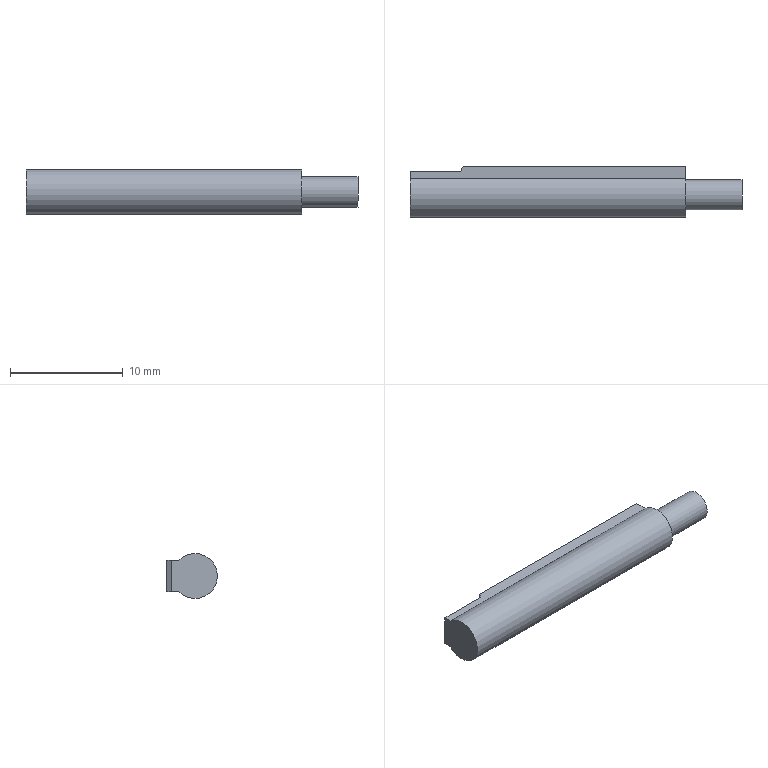Part | NX | 1 solid | 23 faces | box 29.5 x 4.5 x 4 mm | volume 373.823 mm3 | plane 19 | cylinder 4 | commonest cylinder face diameters 2 x1 2.5 x1 2.7 x1 4 x1
STEP:
#1=CARTESIAN_POINT('',(2.462,2.1,-0.8867));
#2=VERTEX_POINT('',#1);
#3=CARTESIAN_POINT('',(1.113,2.1,0.4624));
#4=VERTEX_POINT('',#3);
#5=CARTESIAN_POINT('',(2.,2.1,0.));
#6=DIRECTION('',(0.,1.,0.));
#7=DIRECTION('',(0.,0.,1.));
#8=AXIS2_PLACEMENT_3D('',#5,#6,#7);
#9=CIRCLE('',#8,1.);
#10=EDGE_CURVE('',#2,#4,#9,.T.);
#11=ORIENTED_EDGE('',*,*,#10,.T.);
#12=CARTESIAN_POINT('',(13.738,2.1,-12.162));
#13=DIRECTION('',(0.7071,0.,-0.7071));
#14=VECTOR('',#13,1000.);
#15=LINE('',#12,#14);
#16=EDGE_CURVE('',#4,#2,#15,.T.);
#17=ORIENTED_EDGE('',*,*,#16,.T.);
#18=EDGE_LOOP('',(#11,#17));
#19=FACE_BOUND('',#18,.T.);
#20=CARTESIAN_POINT('',(24.5,2.1,-1.4));
#21=DIRECTION('',(0.,-1.,0.));
#22=DIRECTION('',(0.,0.,-1.));
#23=AXIS2_PLACEMENT_3D('',#20,#21,#22);
#24=PLANE('',#23);
#25=ADVANCED_FACE('',(#19),#24,.F.);
#26=CARTESIAN_POINT('',(24.5,1.428,1.4));
#27=VERTEX_POINT('',#26);
#28=CARTESIAN_POINT('',(24.5,1.428,-1.4));
#29=VERTEX_POINT('',#28);
#30=CARTESIAN_POINT('',(24.5,0.,0.));
#31=DIRECTION('',(1.,0.,0.));
#32=DIRECTION('',(0.,0.,-1.));
#33=AXIS2_PLACEMENT_3D('',#30,#31,#32);
#34=CIRCLE('',#33,2.);
#35=EDGE_CURVE('',#27,#29,#34,.T.);
#36=ORIENTED_EDGE('',*,*,#35,.T.);
#37=CARTESIAN_POINT('',(24.5,2.5,-1.4));
#38=VERTEX_POINT('',#37);
#39=CARTESIAN_POINT('',(24.5,1.428,-1.4));
#40=DIRECTION('',(0.,1.,0.));
#41=VECTOR('',#40,1000.);
#42=LINE('',#39,#41);
#43=EDGE_CURVE('',#29,#38,#42,.T.);
#44=ORIENTED_EDGE('',*,*,#43,.T.);
#45=CARTESIAN_POINT('',(24.5,2.5,1.4));
#46=VERTEX_POINT('',#45);
#47=CARTESIAN_POINT('',(24.5,2.5,1.4));
#48=DIRECTION('',(0.,0.,-1.));
#49=VECTOR('',#48,1000.);
#50=LINE('',#47,#49);
#51=EDGE_CURVE('',#46,#38,#50,.T.);
#52=ORIENTED_EDGE('',*,*,#51,.F.);
#53=CARTESIAN_POINT('',(24.5,2.1,1.4));
#54=DIRECTION('',(0.,-1.,0.));
#55=VECTOR('',#54,1000.);
#56=LINE('',#53,#55);
#57=EDGE_CURVE('',#46,#27,#56,.T.);
#58=ORIENTED_EDGE('',*,*,#57,.T.);
#59=EDGE_LOOP('',(#36,#44,#52,#58));
#60=FACE_BOUND('',#59,.T.);
#61=CARTESIAN_POINT('',(24.5,0.,-1.35));
#62=VERTEX_POINT('',#61);
#63=CARTESIAN_POINT('',(24.5,0.,0.));
#64=DIRECTION('',(1.,0.,0.));
#65=DIRECTION('',(0.,0.,-1.));
#66=AXIS2_PLACEMENT_3D('',#63,#64,#65);
#67=CIRCLE('',#66,1.35);
#68=EDGE_CURVE('',#62,#62,#67,.F.);
#69=ORIENTED_EDGE('',*,*,#68,.T.);
#70=EDGE_LOOP('',(#69));
#71=FACE_BOUND('',#70,.T.);
#72=CARTESIAN_POINT('',(24.5,0.,0.));
#73=DIRECTION('',(1.,0.,0.));
#74=DIRECTION('',(0.,0.,-1.));
#75=AXIS2_PLACEMENT_3D('',#72,#73,#74);
#76=PLANE('',#75);
#77=ADVANCED_FACE('',(#60,#71),#76,.T.);
#78=CARTESIAN_POINT('',(0.,1.428,1.4));
#79=VERTEX_POINT('',#78);
#80=CARTESIAN_POINT('',(0.,1.428,-1.4));
#81=VERTEX_POINT('',#80);
#82=CARTESIAN_POINT('',(0.,0.,0.));
#83=DIRECTION('',(1.,0.,0.));
#84=DIRECTION('',(0.,0.,-1.));
#85=AXIS2_PLACEMENT_3D('',#82,#83,#84);
#86=CIRCLE('',#85,2.);
#87=EDGE_CURVE('',#79,#81,#86,.T.);
#88=ORIENTED_EDGE('',*,*,#87,.T.);
#89=CARTESIAN_POINT('',(24.5,1.428,-1.4));
#90=DIRECTION('',(-1.,0.,0.));
#91=VECTOR('',#90,1000.);
#92=LINE('',#89,#91);
#93=EDGE_CURVE('',#29,#81,#92,.T.);
#94=ORIENTED_EDGE('',*,*,#93,.F.);
#95=ORIENTED_EDGE('',*,*,#35,.F.);
#96=CARTESIAN_POINT('',(24.5,1.428,1.4));
#97=DIRECTION('',(-1.,0.,0.));
#98=VECTOR('',#97,1000.);
#99=LINE('',#96,#98);
#100=EDGE_CURVE('',#27,#79,#99,.T.);
#101=ORIENTED_EDGE('',*,*,#100,.T.);
#102=EDGE_LOOP('',(#88,#94,#95,#101));
#103=FACE_BOUND('',#102,.T.);
#104=CARTESIAN_POINT('',(24.5,0.,0.));
#105=DIRECTION('',(-1.,0.,0.));
#106=DIRECTION('',(0.,0.,1.));
#107=AXIS2_PLACEMENT_3D('',#104,#105,#106);
#108=CYLINDRICAL_SURFACE('',#107,2.);
#109=ADVANCED_FACE('',(#103),#108,.T.);
#110=CARTESIAN_POINT('',(0.,2.1,-1.4));
#111=VERTEX_POINT('',#110);
#112=CARTESIAN_POINT('',(0.,1.428,-1.4));
#113=DIRECTION('',(0.,1.,0.));
#114=VECTOR('',#113,1000.);
#115=LINE('',#112,#114);
#116=EDGE_CURVE('',#81,#111,#115,.T.);
#117=ORIENTED_EDGE('',*,*,#116,.T.);
#118=CARTESIAN_POINT('',(4.5,2.1,-1.4));
#119=VERTEX_POINT('',#118);
#120=CARTESIAN_POINT('',(24.5,2.1,-1.4));
#121=DIRECTION('',(-1.,0.,0.));
#122=VECTOR('',#121,1000.);
#123=LINE('',#120,#122);
#124=EDGE_CURVE('',#119,#111,#123,.T.);
#125=ORIENTED_EDGE('',*,*,#124,.F.);
#126=CARTESIAN_POINT('',(4.731,2.5,-1.4));
#127=VERTEX_POINT('',#126);
#128=CARTESIAN_POINT('',(4.731,2.5,-1.4));
#129=DIRECTION('',(-0.5,-0.866,0.));
#130=VECTOR('',#129,1000.);
#131=LINE('',#128,#130);
#132=EDGE_CURVE('',#127,#119,#131,.T.);
#133=ORIENTED_EDGE('',*,*,#132,.F.);
#134=CARTESIAN_POINT('',(24.5,2.5,-1.4));
#135=DIRECTION('',(-1.,0.,0.));
#136=VECTOR('',#135,1000.);
#137=LINE('',#134,#136);
#138=EDGE_CURVE('',#38,#127,#137,.T.);
#139=ORIENTED_EDGE('',*,*,#138,.F.);
#140=ORIENTED_EDGE('',*,*,#43,.F.);
#141=ORIENTED_EDGE('',*,*,#93,.T.);
#142=EDGE_LOOP('',(#117,#125,#133,#139,#140,#141));
#143=FACE_BOUND('',#142,.T.);
#144=CARTESIAN_POINT('',(24.5,1.428,-1.4));
#145=DIRECTION('',(0.,0.,1.));
#146=DIRECTION('',(1.,0.,0.));
#147=AXIS2_PLACEMENT_3D('',#144,#145,#146);
#148=PLANE('',#147);
#149=ADVANCED_FACE('',(#143),#148,.F.);
#150=CARTESIAN_POINT('',(2.,2.1,1.25));
#151=VERTEX_POINT('',#150);
#152=CARTESIAN_POINT('',(2.,2.1,0.));
#153=DIRECTION('',(0.,1.,0.));
#154=DIRECTION('',(0.,0.,1.));
#155=AXIS2_PLACEMENT_3D('',#152,#153,#154);
#156=CIRCLE('',#155,1.25);
#157=EDGE_CURVE('',#151,#151,#156,.T.);
#158=ORIENTED_EDGE('',*,*,#157,.F.);
#159=EDGE_LOOP('',(#158));
#160=FACE_BOUND('',#159,.T.);
#161=CARTESIAN_POINT('',(4.5,2.1,1.4));
#162=VERTEX_POINT('',#161);
#163=CARTESIAN_POINT('',(0.,2.1,1.4));
#164=VERTEX_POINT('',#163);
#165=CARTESIAN_POINT('',(24.5,2.1,1.4));
#166=DIRECTION('',(-1.,0.,0.));
#167=VECTOR('',#166,1000.);
#168=LINE('',#165,#167);
#169=EDGE_CURVE('',#162,#164,#168,.T.);
#170=ORIENTED_EDGE('',*,*,#169,.F.);
#171=CARTESIAN_POINT('',(4.5,2.1,1.4));
#172=DIRECTION('',(0.,0.,-1.));
#173=VECTOR('',#172,1000.);
#174=LINE('',#171,#173);
#175=EDGE_CURVE('',#162,#119,#174,.T.);
#176=ORIENTED_EDGE('',*,*,#175,.T.);
#177=ORIENTED_EDGE('',*,*,#124,.T.);
#178=CARTESIAN_POINT('',(0.,2.1,-1.4));
#179=DIRECTION('',(0.,0.,1.));
#180=VECTOR('',#179,1000.);
#181=LINE('',#178,#180);
#182=EDGE_CURVE('',#111,#164,#181,.T.);
#183=ORIENTED_EDGE('',*,*,#182,.T.);
#184=EDGE_LOOP('',(#170,#176,#177,#183));
#185=FACE_BOUND('',#184,.T.);
#186=CARTESIAN_POINT('',(24.5,2.1,-1.4));
#187=DIRECTION('',(0.,-1.,0.));
#188=DIRECTION('',(0.,0.,-1.));
#189=AXIS2_PLACEMENT_3D('',#186,#187,#188);
#190=PLANE('',#189);
#191=ADVANCED_FACE('',(#160,#185),#190,.F.);
#192=CARTESIAN_POINT('',(0.,2.1,1.4));
#193=DIRECTION('',(0.,-1.,0.));
#194=VECTOR('',#193,1000.);
#195=LINE('',#192,#194);
#196=EDGE_CURVE('',#164,#79,#195,.T.);
#197=ORIENTED_EDGE('',*,*,#196,.T.);
#198=ORIENTED_EDGE('',*,*,#100,.F.);
#199=ORIENTED_EDGE('',*,*,#57,.F.);
#200=CARTESIAN_POINT('',(4.731,2.5,1.4));
#201=VERTEX_POINT('',#200);
#202=CARTESIAN_POINT('',(24.5,2.5,1.4));
#203=DIRECTION('',(-1.,0.,0.));
#204=VECTOR('',#203,1000.);
#205=LINE('',#202,#204);
#206=EDGE_CURVE('',#46,#201,#205,.T.);
#207=ORIENTED_EDGE('',*,*,#206,.T.);
#208=CARTESIAN_POINT('',(4.731,2.5,1.4));
#209=DIRECTION('',(-0.5,-0.866,0.));
#210=VECTOR('',#209,1000.);
#211=LINE('',#208,#210);
#212=EDGE_CURVE('',#201,#162,#211,.T.);
#213=ORIENTED_EDGE('',*,*,#212,.T.);
#214=ORIENTED_EDGE('',*,*,#169,.T.);
#215=EDGE_LOOP('',(#197,#198,#199,#207,#213,#214));
#216=FACE_BOUND('',#215,.T.);
#217=CARTESIAN_POINT('',(24.5,2.1,1.4));
#218=DIRECTION('',(0.,0.,-1.));
#219=DIRECTION('',(-1.,0.,0.));
#220=AXIS2_PLACEMENT_3D('',#217,#218,#219);
#221=PLANE('',#220);
#222=ADVANCED_FACE('',(#216),#221,.F.);
#223=ORIENTED_EDGE('',*,*,#87,.F.);
#224=ORIENTED_EDGE('',*,*,#196,.F.);
#225=ORIENTED_EDGE('',*,*,#182,.F.);
#226=ORIENTED_EDGE('',*,*,#116,.F.);
#227=EDGE_LOOP('',(#223,#224,#225,#226));
#228=FACE_BOUND('',#227,.T.);
#229=CARTESIAN_POINT('',(0.,0.,0.));
#230=DIRECTION('',(1.,0.,0.));
#231=DIRECTION('',(0.,0.,-1.));
#232=AXIS2_PLACEMENT_3D('',#229,#230,#231);
#233=PLANE('',#232);
#234=ADVANCED_FACE('',(#228),#233,.F.);
#235=ORIENTED_EDGE('',*,*,#68,.F.);
#236=EDGE_LOOP('',(#235));
#237=FACE_BOUND('',#236,.T.);
#238=CARTESIAN_POINT('',(29.5,0.,-1.35));
#239=VERTEX_POINT('',#238);
#240=CARTESIAN_POINT('',(29.5,0.,0.));
#241=DIRECTION('',(1.,0.,0.));
#242=DIRECTION('',(0.,0.,-1.));
#243=AXIS2_PLACEMENT_3D('',#240,#241,#242);
#244=CIRCLE('',#243,1.35);
#245=EDGE_CURVE('',#239,#239,#244,.T.);
#246=ORIENTED_EDGE('',*,*,#245,.F.);
#247=EDGE_LOOP('',(#246));
#248=FACE_BOUND('',#247,.T.);
#249=CARTESIAN_POINT('',(29.5,0.,0.));
#250=DIRECTION('',(-1.,0.,0.));
#251=DIRECTION('',(0.,0.,1.));
#252=AXIS2_PLACEMENT_3D('',#249,#250,#251);
#253=CYLINDRICAL_SURFACE('',#252,1.35);
#254=ADVANCED_FACE('',(#237,#248),#253,.T.);
#255=ORIENTED_EDGE('',*,*,#245,.T.);
#256=EDGE_LOOP('',(#255));
#257=FACE_BOUND('',#256,.T.);
#258=CARTESIAN_POINT('',(29.5,0.,0.));
#259=DIRECTION('',(1.,0.,0.));
#260=DIRECTION('',(0.,0.,-1.));
#261=AXIS2_PLACEMENT_3D('',#258,#259,#260);
#262=PLANE('',#261);
#263=ADVANCED_FACE('',(#257),#262,.T.);
#264=CARTESIAN_POINT('',(2.,0.6,1.25));
#265=VERTEX_POINT('',#264);
#266=CARTESIAN_POINT('',(2.,0.6,0.));
#267=DIRECTION('',(0.,1.,0.));
#268=DIRECTION('',(0.,0.,1.));
#269=AXIS2_PLACEMENT_3D('',#266,#267,#268);
#270=CIRCLE('',#269,1.25);
#271=EDGE_CURVE('',#265,#265,#270,.T.);
#272=ORIENTED_EDGE('',*,*,#271,.F.);
#273=EDGE_LOOP('',(#272));
#274=FACE_BOUND('',#273,.T.);
#275=ORIENTED_EDGE('',*,*,#157,.T.);
#276=EDGE_LOOP('',(#275));
#277=FACE_BOUND('',#276,.T.);
#278=CARTESIAN_POINT('',(2.,0.6,0.));
#279=DIRECTION('',(0.,1.,0.));
#280=DIRECTION('',(0.,0.,1.));
#281=AXIS2_PLACEMENT_3D('',#278,#279,#280);
#282=CYLINDRICAL_SURFACE('',#281,1.25);
#283=ADVANCED_FACE('',(#274,#277),#282,.F.);
#284=CARTESIAN_POINT('',(2.,0.6,1.));
#285=VERTEX_POINT('',#284);
#286=CARTESIAN_POINT('',(2.,0.6,0.));
#287=DIRECTION('',(0.,1.,0.));
#288=DIRECTION('',(0.,0.,1.));
#289=AXIS2_PLACEMENT_3D('',#286,#287,#288);
#290=CIRCLE('',#289,1.);
#291=EDGE_CURVE('',#285,#285,#290,.T.);
#292=ORIENTED_EDGE('',*,*,#291,.F.);
#293=EDGE_LOOP('',(#292));
#294=FACE_BOUND('',#293,.T.);
#295=ORIENTED_EDGE('',*,*,#271,.T.);
#296=EDGE_LOOP('',(#295));
#297=FACE_BOUND('',#296,.T.);
#298=CARTESIAN_POINT('',(2.,0.6,0.));
#299=DIRECTION('',(0.,1.,0.));
#300=DIRECTION('',(0.,0.,1.));
#301=AXIS2_PLACEMENT_3D('',#298,#299,#300);
#302=PLANE('',#301);
#303=ADVANCED_FACE('',(#294,#297),#302,.T.);
#304=CARTESIAN_POINT('',(1.113,1.1,0.4624));
#305=VERTEX_POINT('',#304);
#306=CARTESIAN_POINT('',(1.113,0.6,0.4624));
#307=DIRECTION('',(0.,1.,0.));
#308=VECTOR('',#307,1000.);
#309=LINE('',#306,#308);
#310=EDGE_CURVE('',#4,#305,#309,.F.);
#311=ORIENTED_EDGE('',*,*,#310,.F.);
#312=ORIENTED_EDGE('',*,*,#10,.F.);
#313=CARTESIAN_POINT('',(2.462,1.1,-0.8867));
#314=VERTEX_POINT('',#313);
#315=CARTESIAN_POINT('',(2.462,0.6,-0.8867));
#316=DIRECTION('',(0.,1.,0.));
#317=VECTOR('',#316,1000.);
#318=LINE('',#315,#317);
#319=EDGE_CURVE('',#314,#2,#318,.T.);
#320=ORIENTED_EDGE('',*,*,#319,.F.);
#321=CARTESIAN_POINT('',(2.887,1.1,-0.4624));
#322=VERTEX_POINT('',#321);
#323=CARTESIAN_POINT('',(2.,1.1,0.));
#324=DIRECTION('',(0.,1.,0.));
#325=DIRECTION('',(0.,0.,1.));
#326=AXIS2_PLACEMENT_3D('',#323,#324,#325);
#327=CIRCLE('',#326,1.);
#328=EDGE_CURVE('',#314,#322,#327,.F.);
#329=ORIENTED_EDGE('',*,*,#328,.T.);
#330=CARTESIAN_POINT('',(2.887,2.1,-0.4624));
#331=VERTEX_POINT('',#330);
#332=CARTESIAN_POINT('',(2.887,0.6,-0.4624));
#333=DIRECTION('',(0.,1.,0.));
#334=VECTOR('',#333,1000.);
#335=LINE('',#332,#334);
#336=EDGE_CURVE('',#331,#322,#335,.F.);
#337=ORIENTED_EDGE('',*,*,#336,.F.);
#338=CARTESIAN_POINT('',(1.538,2.1,0.8867));
#339=VERTEX_POINT('',#338);
#340=CARTESIAN_POINT('',(2.,2.1,0.));
#341=DIRECTION('',(0.,1.,0.));
#342=DIRECTION('',(0.,0.,1.));
#343=AXIS2_PLACEMENT_3D('',#340,#341,#342);
#344=CIRCLE('',#343,1.);
#345=EDGE_CURVE('',#339,#331,#344,.T.);
#346=ORIENTED_EDGE('',*,*,#345,.F.);
#347=CARTESIAN_POINT('',(1.538,1.1,0.8867));
#348=VERTEX_POINT('',#347);
#349=CARTESIAN_POINT('',(1.538,0.6,0.8867));
#350=DIRECTION('',(0.,1.,0.));
#351=VECTOR('',#350,1000.);
#352=LINE('',#349,#351);
#353=EDGE_CURVE('',#348,#339,#352,.T.);
#354=ORIENTED_EDGE('',*,*,#353,.F.);
#355=CARTESIAN_POINT('',(2.,1.1,0.));
#356=DIRECTION('',(0.,1.,0.));
#357=DIRECTION('',(0.,0.,1.));
#358=AXIS2_PLACEMENT_3D('',#355,#356,#357);
#359=CIRCLE('',#358,1.);
#360=EDGE_CURVE('',#348,#305,#359,.F.);
#361=ORIENTED_EDGE('',*,*,#360,.T.);
#362=EDGE_LOOP('',(#311,#312,#320,#329,#337,#346,#354,#361));
#363=FACE_BOUND('',#362,.T.);
#364=ORIENTED_EDGE('',*,*,#291,.T.);
#365=EDGE_LOOP('',(#364));
#366=FACE_BOUND('',#365,.T.);
#367=CARTESIAN_POINT('',(2.,0.6,0.));
#368=DIRECTION('',(0.,1.,0.));
#369=DIRECTION('',(0.,0.,1.));
#370=AXIS2_PLACEMENT_3D('',#367,#368,#369);
#371=CYLINDRICAL_SURFACE('',#370,1.);
#372=ADVANCED_FACE('',(#363,#366),#371,.T.);
#373=ORIENTED_EDGE('',*,*,#345,.T.);
#374=CARTESIAN_POINT('',(14.162,2.1,-11.738));
#375=DIRECTION('',(-0.7071,0.,0.7071));
#376=VECTOR('',#375,1000.);
#377=LINE('',#374,#376);
#378=EDGE_CURVE('',#331,#339,#377,.T.);
#379=ORIENTED_EDGE('',*,*,#378,.T.);
#380=EDGE_LOOP('',(#373,#379));
#381=FACE_BOUND('',#380,.T.);
#382=CARTESIAN_POINT('',(24.5,2.1,-1.4));
#383=DIRECTION('',(0.,-1.,0.));
#384=DIRECTION('',(0.,0.,-1.));
#385=AXIS2_PLACEMENT_3D('',#382,#383,#384);
#386=PLANE('',#385);
#387=ADVANCED_FACE('',(#381),#386,.F.);
#388=ORIENTED_EDGE('',*,*,#310,.T.);
#389=CARTESIAN_POINT('',(2.536,1.1,-0.9605));
#390=DIRECTION('',(-0.7071,0.,0.7071));
#391=VECTOR('',#390,1000.);
#392=LINE('',#389,#391);
#393=EDGE_CURVE('',#314,#305,#392,.T.);
#394=ORIENTED_EDGE('',*,*,#393,.F.);
#395=ORIENTED_EDGE('',*,*,#319,.T.);
#396=ORIENTED_EDGE('',*,*,#16,.F.);
#397=EDGE_LOOP('',(#388,#394,#395,#396));
#398=FACE_BOUND('',#397,.T.);
#399=CARTESIAN_POINT('',(2.536,1.1,-0.9605));
#400=DIRECTION('',(-0.7071,0.,-0.7071));
#401=DIRECTION('',(-0.7071,0.,0.7071));
#402=AXIS2_PLACEMENT_3D('',#399,#400,#401);
#403=PLANE('',#402);
#404=ADVANCED_FACE('',(#398),#403,.F.);
#405=ORIENTED_EDGE('',*,*,#336,.T.);
#406=CARTESIAN_POINT('',(1.464,1.1,0.9605));
#407=DIRECTION('',(0.7071,0.,-0.7071));
#408=VECTOR('',#407,1000.);
#409=LINE('',#406,#408);
#410=EDGE_CURVE('',#348,#322,#409,.T.);
#411=ORIENTED_EDGE('',*,*,#410,.F.);
#412=ORIENTED_EDGE('',*,*,#353,.T.);
#413=ORIENTED_EDGE('',*,*,#378,.F.);
#414=EDGE_LOOP('',(#405,#411,#412,#413));
#415=FACE_BOUND('',#414,.T.);
#416=CARTESIAN_POINT('',(1.464,1.1,0.9605));
#417=DIRECTION('',(0.7071,0.,0.7071));
#418=DIRECTION('',(0.7071,0.,-0.7071));
#419=AXIS2_PLACEMENT_3D('',#416,#417,#418);
#420=PLANE('',#419);
#421=ADVANCED_FACE('',(#415),#420,.F.);
#422=ORIENTED_EDGE('',*,*,#410,.T.);
#423=ORIENTED_EDGE('',*,*,#328,.F.);
#424=ORIENTED_EDGE('',*,*,#393,.T.);
#425=ORIENTED_EDGE('',*,*,#360,.F.);
#426=EDGE_LOOP('',(#422,#423,#424,#425));
#427=FACE_BOUND('',#426,.T.);
#428=CARTESIAN_POINT('',(2.,1.1,0.));
#429=DIRECTION('',(0.,1.,0.));
#430=DIRECTION('',(0.,0.,1.));
#431=AXIS2_PLACEMENT_3D('',#428,#429,#430);
#432=PLANE('',#431);
#433=ADVANCED_FACE('',(#427),#432,.T.);
#434=CARTESIAN_POINT('',(4.731,2.5,1.4));
#435=DIRECTION('',(0.,0.,-1.));
#436=VECTOR('',#435,1000.);
#437=LINE('',#434,#436);
#438=EDGE_CURVE('',#201,#127,#437,.T.);
#439=ORIENTED_EDGE('',*,*,#438,.T.);
#440=ORIENTED_EDGE('',*,*,#132,.T.);
#441=ORIENTED_EDGE('',*,*,#175,.F.);
#442=ORIENTED_EDGE('',*,*,#212,.F.);
#443=EDGE_LOOP('',(#439,#440,#441,#442));
#444=FACE_BOUND('',#443,.T.);
#445=CARTESIAN_POINT('',(4.731,2.5,1.4));
#446=DIRECTION('',(0.866,-0.5,0.));
#447=DIRECTION('',(0.5,0.866,0.));
#448=AXIS2_PLACEMENT_3D('',#445,#446,#447);
#449=PLANE('',#448);
#450=ADVANCED_FACE('',(#444),#449,.F.);
#451=CARTESIAN_POINT('',(6.5,2.5,0.5));
#452=VERTEX_POINT('',#451);
#453=CARTESIAN_POINT('',(7.5,2.5,0.5));
#454=VERTEX_POINT('',#453);
#455=CARTESIAN_POINT('',(6.5,2.5,0.5));
#456=DIRECTION('',(1.,0.,0.));
#457=VECTOR('',#456,1000.);
#458=LINE('',#455,#457);
#459=EDGE_CURVE('',#452,#454,#458,.T.);
#460=ORIENTED_EDGE('',*,*,#459,.F.);
#461=CARTESIAN_POINT('',(6.5,2.5,-0.5));
#462=VERTEX_POINT('',#461);
#463=CARTESIAN_POINT('',(6.5,2.5,-0.5));
#464=DIRECTION('',(0.,0.,1.));
#465=VECTOR('',#464,1000.);
#466=LINE('',#463,#465);
#467=EDGE_CURVE('',#462,#452,#466,.T.);
#468=ORIENTED_EDGE('',*,*,#467,.F.);
#469=CARTESIAN_POINT('',(7.5,2.5,-0.5));
#470=VERTEX_POINT('',#469);
#471=CARTESIAN_POINT('',(7.5,2.5,-0.5));
#472=DIRECTION('',(-1.,0.,0.));
#473=VECTOR('',#472,1000.);
#474=LINE('',#471,#473);
#475=EDGE_CURVE('',#470,#462,#474,.T.);
#476=ORIENTED_EDGE('',*,*,#475,.F.);
#477=CARTESIAN_POINT('',(7.5,2.5,0.5));
#478=DIRECTION('',(0.,0.,-1.));
#479=VECTOR('',#478,1000.);
#480=LINE('',#477,#479);
#481=EDGE_CURVE('',#454,#470,#480,.T.);
#482=ORIENTED_EDGE('',*,*,#481,.F.);
#483=EDGE_LOOP('',(#460,#468,#476,#482));
#484=FACE_BOUND('',#483,.T.);
#485=ORIENTED_EDGE('',*,*,#51,.T.);
#486=ORIENTED_EDGE('',*,*,#138,.T.);
#487=ORIENTED_EDGE('',*,*,#438,.F.);
#488=ORIENTED_EDGE('',*,*,#206,.F.);
#489=EDGE_LOOP('',(#485,#486,#487,#488));
#490=FACE_BOUND('',#489,.T.);
#491=CARTESIAN_POINT('',(24.5,2.5,1.4));
#492=DIRECTION('',(0.,-1.,0.));
#493=DIRECTION('',(0.,0.,-1.));
#494=AXIS2_PLACEMENT_3D('',#491,#492,#493);
#495=PLANE('',#494);
#496=ADVANCED_FACE('',(#484,#490),#495,.F.);
#497=ORIENTED_EDGE('',*,*,#467,.T.);
#498=CARTESIAN_POINT('',(6.5,2.3,0.5));
#499=VERTEX_POINT('',#498);
#500=CARTESIAN_POINT('',(6.5,2.3,0.5));
#501=DIRECTION('',(0.,1.,0.));
#502=VECTOR('',#501,1000.);
#503=LINE('',#500,#502);
#504=EDGE_CURVE('',#499,#452,#503,.T.);
#505=ORIENTED_EDGE('',*,*,#504,.F.);
#506=CARTESIAN_POINT('',(6.5,2.3,-0.5));
#507=VERTEX_POINT('',#506);
#508=CARTESIAN_POINT('',(6.5,2.3,-0.5));
#509=DIRECTION('',(0.,0.,1.));
#510=VECTOR('',#509,1000.);
#511=LINE('',#508,#510);
#512=EDGE_CURVE('',#507,#499,#511,.T.);
#513=ORIENTED_EDGE('',*,*,#512,.F.);
#514=CARTESIAN_POINT('',(6.5,2.3,-0.5));
#515=DIRECTION('',(0.,1.,0.));
#516=VECTOR('',#515,1000.);
#517=LINE('',#514,#516);
#518=EDGE_CURVE('',#507,#462,#517,.T.);
#519=ORIENTED_EDGE('',*,*,#518,.T.);
#520=EDGE_LOOP('',(#497,#505,#513,#519));
#521=FACE_BOUND('',#520,.T.);
#522=CARTESIAN_POINT('',(6.5,2.3,-0.5));
#523=DIRECTION('',(-1.,0.,0.));
#524=DIRECTION('',(0.,0.,1.));
#525=AXIS2_PLACEMENT_3D('',#522,#523,#524);
#526=PLANE('',#525);
#527=ADVANCED_FACE('',(#521),#526,.F.);
#528=ORIENTED_EDGE('',*,*,#475,.T.);
#529=ORIENTED_EDGE('',*,*,#518,.F.);
#530=CARTESIAN_POINT('',(7.5,2.3,-0.5));
#531=VERTEX_POINT('',#530);
#532=CARTESIAN_POINT('',(7.5,2.3,-0.5));
#533=DIRECTION('',(-1.,0.,0.));
#534=VECTOR('',#533,1000.);
#535=LINE('',#532,#534);
#536=EDGE_CURVE('',#531,#507,#535,.T.);
#537=ORIENTED_EDGE('',*,*,#536,.F.);
#538=CARTESIAN_POINT('',(7.5,2.3,-0.5));
#539=DIRECTION('',(0.,1.,0.));
#540=VECTOR('',#539,1000.);
#541=LINE('',#538,#540);
#542=EDGE_CURVE('',#531,#470,#541,.T.);
#543=ORIENTED_EDGE('',*,*,#542,.T.);
#544=EDGE_LOOP('',(#528,#529,#537,#543));
#545=FACE_BOUND('',#544,.T.);
#546=CARTESIAN_POINT('',(7.5,2.3,-0.5));
#547=DIRECTION('',(0.,0.,-1.));
#548=DIRECTION('',(-1.,0.,0.));
#549=AXIS2_PLACEMENT_3D('',#546,#547,#548);
#550=PLANE('',#549);
#551=ADVANCED_FACE('',(#545),#550,.F.);
#552=ORIENTED_EDGE('',*,*,#481,.T.);
#553=ORIENTED_EDGE('',*,*,#542,.F.);
#554=CARTESIAN_POINT('',(7.5,2.3,0.5));
#555=VERTEX_POINT('',#554);
#556=CARTESIAN_POINT('',(7.5,2.3,0.5));
#557=DIRECTION('',(0.,0.,-1.));
#558=VECTOR('',#557,1000.);
#559=LINE('',#556,#558);
#560=EDGE_CURVE('',#555,#531,#559,.T.);
#561=ORIENTED_EDGE('',*,*,#560,.F.);
#562=CARTESIAN_POINT('',(7.5,2.3,0.5));
#563=DIRECTION('',(0.,1.,0.));
#564=VECTOR('',#563,1000.);
#565=LINE('',#562,#564);
#566=EDGE_CURVE('',#555,#454,#565,.T.);
#567=ORIENTED_EDGE('',*,*,#566,.T.);
#568=EDGE_LOOP('',(#552,#553,#561,#567));
#569=FACE_BOUND('',#568,.T.);
#570=CARTESIAN_POINT('',(7.5,2.3,0.5));
#571=DIRECTION('',(1.,0.,0.));
#572=DIRECTION('',(0.,0.,-1.));
#573=AXIS2_PLACEMENT_3D('',#570,#571,#572);
#574=PLANE('',#573);
#575=ADVANCED_FACE('',(#569),#574,.F.);
#576=ORIENTED_EDGE('',*,*,#459,.T.);
#577=ORIENTED_EDGE('',*,*,#566,.F.);
#578=CARTESIAN_POINT('',(6.5,2.3,0.5));
#579=DIRECTION('',(1.,0.,0.));
#580=VECTOR('',#579,1000.);
#581=LINE('',#578,#580);
#582=EDGE_CURVE('',#499,#555,#581,.T.);
#583=ORIENTED_EDGE('',*,*,#582,.F.);
#584=ORIENTED_EDGE('',*,*,#504,.T.);
#585=EDGE_LOOP('',(#576,#577,#583,#584));
#586=FACE_BOUND('',#585,.T.);
#587=CARTESIAN_POINT('',(6.5,2.3,0.5));
#588=DIRECTION('',(0.,0.,1.));
#589=DIRECTION('',(1.,0.,0.));
#590=AXIS2_PLACEMENT_3D('',#587,#588,#589);
#591=PLANE('',#590);
#592=ADVANCED_FACE('',(#586),#591,.F.);
#593=ORIENTED_EDGE('',*,*,#512,.T.);
#594=ORIENTED_EDGE('',*,*,#582,.T.);
#595=ORIENTED_EDGE('',*,*,#560,.T.);
#596=ORIENTED_EDGE('',*,*,#536,.T.);
#597=EDGE_LOOP('',(#593,#594,#595,#596));
#598=FACE_BOUND('',#597,.T.);
#599=CARTESIAN_POINT('',(0.,2.3,0.));
#600=DIRECTION('',(0.,1.,0.));
#601=DIRECTION('',(0.,0.,1.));
#602=AXIS2_PLACEMENT_3D('',#599,#600,#601);
#603=PLANE('',#602);
#604=ADVANCED_FACE('',(#598),#603,.T.);
#605=CLOSED_SHELL('',(#25,#77,#109,#149,#191,#222,#234,#254,#263,#283,#303,#372,#387,#404,#421,#433,#450,#496,#527,#551,#575,#592,#604));
#606=MANIFOLD_SOLID_BREP('',#605);
#607=(LENGTH_UNIT()NAMED_UNIT(*)SI_UNIT(.MILLI.,.METRE.));
#608=UNCERTAINTY_MEASURE_WITH_UNIT(LENGTH_MEASURE(0.00001),#607,'','');
#609=(NAMED_UNIT(*)PLANE_ANGLE_UNIT()SI_UNIT($,.RADIAN.));
#610=(NAMED_UNIT(*)SI_UNIT($,.STERADIAN.)SOLID_ANGLE_UNIT());
#611=(GEOMETRIC_REPRESENTATION_CONTEXT(3)GLOBAL_UNCERTAINTY_ASSIGNED_CONTEXT((#608))GLOBAL_UNIT_ASSIGNED_CONTEXT((#607,#609,#610))REPRESENTATION_CONTEXT('',''));
#612=ADVANCED_BREP_SHAPE_REPRESENTATION('',(#606),#611);